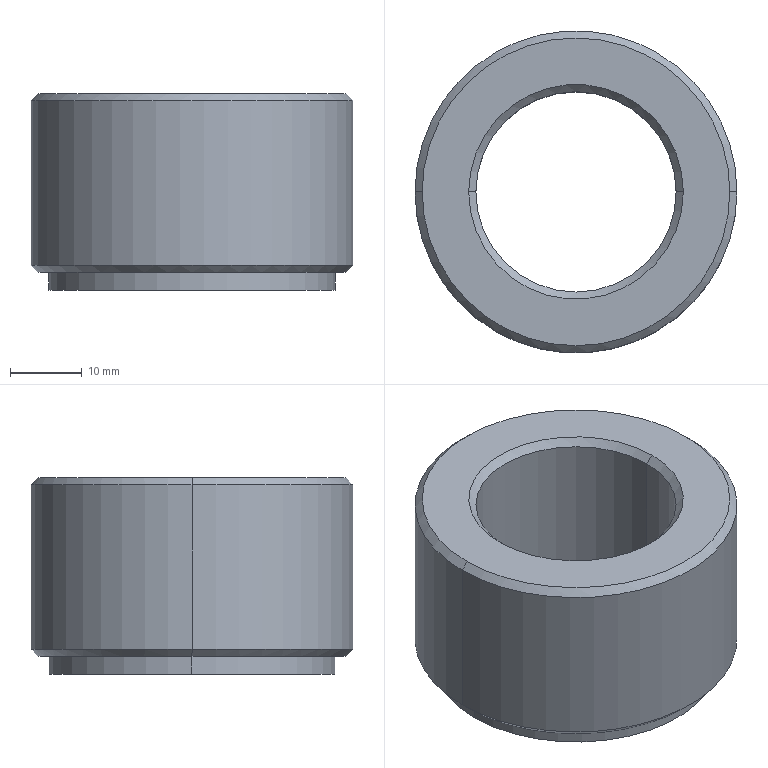Part | SolidWorks | features 3DProfileFeature 1, Chamfer 1, Extrusion 1, HoleWzd 1, ICE 1 | 1 solid | 15 faces | box 45 x 45 x 27.5 mm | volume 25785 mm3 | cone 6 | cylinder 6 | plane 3 | commonest cylinder face diameters 28 x2 40 x2 45 x2
STEP:
#1=CARTESIAN_POINT('',(-83.421,0.,24.));
#2=VERTEX_POINT('',#1);
#3=CARTESIAN_POINT('',(-55.421,0.,24.));
#4=VERTEX_POINT('',#3);
#5=CARTESIAN_POINT('',(-69.421,0.,24.));
#6=DIRECTION('',(0.,0.,1.));
#7=DIRECTION('',(1.,0.,0.));
#8=AXIS2_PLACEMENT_3D('',#5,#6,#7);
#9=CIRCLE('',#8,14.);
#10=EDGE_CURVE('',#2,#4,#9,.T.);
#11=ORIENTED_EDGE('',*,*,#10,.F.);
#12=CARTESIAN_POINT('',(-84.421,0.,25.));
#13=VERTEX_POINT('',#12);
#14=CARTESIAN_POINT('',(-83.421,0.,24.));
#15=DIRECTION('',(-0.7071,0.,0.7071));
#16=VECTOR('',#15,1000.);
#17=LINE('',#14,#16);
#18=EDGE_CURVE('',#2,#13,#17,.T.);
#19=ORIENTED_EDGE('',*,*,#18,.T.);
#20=CARTESIAN_POINT('',(-54.421,0.,25.));
#21=VERTEX_POINT('',#20);
#22=CARTESIAN_POINT('',(-69.421,0.,25.));
#23=DIRECTION('',(0.,0.,-1.));
#24=DIRECTION('',(1.,0.,0.));
#25=AXIS2_PLACEMENT_3D('',#22,#23,#24);
#26=CIRCLE('',#25,15.);
#27=EDGE_CURVE('',#21,#13,#26,.T.);
#28=ORIENTED_EDGE('',*,*,#27,.F.);
#29=CARTESIAN_POINT('',(-55.421,0.,24.));
#30=DIRECTION('',(0.7071,0.,0.7071));
#31=VECTOR('',#30,1000.);
#32=LINE('',#29,#31);
#33=EDGE_CURVE('',#4,#21,#32,.T.);
#34=ORIENTED_EDGE('',*,*,#33,.F.);
#35=EDGE_LOOP('',(#11,#19,#28,#34));
#36=FACE_OUTER_BOUND('',#35,.T.);
#37=CARTESIAN_POINT('',(-69.421,0.,24.));
#38=DIRECTION('',(0.,0.,1.));
#39=DIRECTION('',(1.,0.,0.));
#40=AXIS2_PLACEMENT_3D('',#37,#38,#39);
#41=CONICAL_SURFACE('',#40,14.,0.7854);
#42=ADVANCED_FACE('',(#36),#41,.F.);
#43=CARTESIAN_POINT('',(-47.921,0.,25.));
#44=VERTEX_POINT('',#43);
#45=CARTESIAN_POINT('',(-90.921,0.,25.));
#46=VERTEX_POINT('',#45);
#47=CARTESIAN_POINT('',(-69.421,0.,25.));
#48=DIRECTION('',(0.,0.,1.));
#49=DIRECTION('',(1.,0.,0.));
#50=AXIS2_PLACEMENT_3D('',#47,#48,#49);
#51=CIRCLE('',#50,21.5);
#52=EDGE_CURVE('',#44,#46,#51,.T.);
#53=ORIENTED_EDGE('',*,*,#52,.F.);
#54=CARTESIAN_POINT('',(-46.921,0.,24.));
#55=VERTEX_POINT('',#54);
#56=CARTESIAN_POINT('',(-47.921,0.,25.));
#57=DIRECTION('',(0.7071,0.,-0.7071));
#58=VECTOR('',#57,1000.);
#59=LINE('',#56,#58);
#60=EDGE_CURVE('',#44,#55,#59,.T.);
#61=ORIENTED_EDGE('',*,*,#60,.T.);
#62=CARTESIAN_POINT('',(-91.921,0.,24.));
#63=VERTEX_POINT('',#62);
#64=CARTESIAN_POINT('',(-69.421,0.,24.));
#65=DIRECTION('',(0.,0.,-1.));
#66=DIRECTION('',(1.,0.,0.));
#67=AXIS2_PLACEMENT_3D('',#64,#65,#66);
#68=CIRCLE('',#67,22.5);
#69=EDGE_CURVE('',#63,#55,#68,.T.);
#70=ORIENTED_EDGE('',*,*,#69,.F.);
#71=CARTESIAN_POINT('',(-90.921,0.,25.));
#72=DIRECTION('',(-0.7071,0.,-0.7071));
#73=VECTOR('',#72,1000.);
#74=LINE('',#71,#73);
#75=EDGE_CURVE('',#46,#63,#74,.T.);
#76=ORIENTED_EDGE('',*,*,#75,.F.);
#77=EDGE_LOOP('',(#53,#61,#70,#76));
#78=FACE_OUTER_BOUND('',#77,.T.);
#79=CARTESIAN_POINT('',(-69.421,0.,25.));
#80=DIRECTION('',(0.,0.,-1.));
#81=DIRECTION('',(-1.,0.,0.));
#82=AXIS2_PLACEMENT_3D('',#79,#80,#81);
#83=CONICAL_SURFACE('',#82,21.5,0.7854);
#84=ADVANCED_FACE('',(#78),#83,.T.);
#85=CARTESIAN_POINT('',(-90.921,0.,0.));
#86=VERTEX_POINT('',#85);
#87=CARTESIAN_POINT('',(-47.921,0.,0.));
#88=VERTEX_POINT('',#87);
#89=CARTESIAN_POINT('',(-69.421,0.,0.));
#90=DIRECTION('',(0.,0.,-1.));
#91=DIRECTION('',(1.,0.,0.));
#92=AXIS2_PLACEMENT_3D('',#89,#90,#91);
#93=CIRCLE('',#92,21.5);
#94=EDGE_CURVE('',#86,#88,#93,.T.);
#95=ORIENTED_EDGE('',*,*,#94,.F.);
#96=CARTESIAN_POINT('',(-91.921,0.,1.));
#97=VERTEX_POINT('',#96);
#98=CARTESIAN_POINT('',(-91.921,0.,1.));
#99=DIRECTION('',(-0.7071,0.,0.7071));
#100=VECTOR('',#99,1000.);
#101=LINE('',#98,#100);
#102=EDGE_CURVE('',#86,#97,#101,.T.);
#103=ORIENTED_EDGE('',*,*,#102,.T.);
#104=CARTESIAN_POINT('',(-46.921,0.,1.));
#105=VERTEX_POINT('',#104);
#106=CARTESIAN_POINT('',(-69.421,0.,1.));
#107=DIRECTION('',(0.,0.,1.));
#108=DIRECTION('',(1.,0.,0.));
#109=AXIS2_PLACEMENT_3D('',#106,#107,#108);
#110=CIRCLE('',#109,22.5);
#111=EDGE_CURVE('',#105,#97,#110,.T.);
#112=ORIENTED_EDGE('',*,*,#111,.F.);
#113=CARTESIAN_POINT('',(-46.921,0.,1.));
#114=DIRECTION('',(0.7071,0.,0.7071));
#115=VECTOR('',#114,1000.);
#116=LINE('',#113,#115);
#117=EDGE_CURVE('',#88,#105,#116,.T.);
#118=ORIENTED_EDGE('',*,*,#117,.F.);
#119=EDGE_LOOP('',(#95,#103,#112,#118));
#120=FACE_OUTER_BOUND('',#119,.T.);
#121=CARTESIAN_POINT('',(-69.421,0.,1.));
#122=DIRECTION('',(0.,0.,1.));
#123=DIRECTION('',(1.,0.,0.));
#124=AXIS2_PLACEMENT_3D('',#121,#122,#123);
#125=CONICAL_SURFACE('',#124,22.5,0.7854);
#126=ADVANCED_FACE('',(#120),#125,.T.);
#127=CARTESIAN_POINT('',(-89.421,0.,-2.5));
#128=VERTEX_POINT('',#127);
#129=CARTESIAN_POINT('',(-49.421,0.,-2.5));
#130=VERTEX_POINT('',#129);
#131=CARTESIAN_POINT('',(-69.421,0.,-2.5));
#132=DIRECTION('',(0.,0.,-1.));
#133=DIRECTION('',(-1.,0.,0.));
#134=AXIS2_PLACEMENT_3D('',#131,#132,#133);
#135=CIRCLE('',#134,20.);
#136=EDGE_CURVE('',#128,#130,#135,.T.);
#137=ORIENTED_EDGE('',*,*,#136,.F.);
#138=CARTESIAN_POINT('',(-89.421,0.,0.));
#139=VERTEX_POINT('',#138);
#140=CARTESIAN_POINT('',(-89.421,0.,-2.5));
#141=DIRECTION('',(0.,0.,1.));
#142=VECTOR('',#141,1000.);
#143=LINE('',#140,#142);
#144=EDGE_CURVE('',#128,#139,#143,.T.);
#145=ORIENTED_EDGE('',*,*,#144,.T.);
#146=CARTESIAN_POINT('',(-49.421,0.,0.));
#147=VERTEX_POINT('',#146);
#148=CARTESIAN_POINT('',(-69.421,0.,0.));
#149=DIRECTION('',(0.,0.,-1.));
#150=DIRECTION('',(1.,0.,0.));
#151=AXIS2_PLACEMENT_3D('',#148,#149,#150);
#152=CIRCLE('',#151,20.);
#153=EDGE_CURVE('',#139,#147,#152,.T.);
#154=ORIENTED_EDGE('',*,*,#153,.T.);
#155=CARTESIAN_POINT('',(-49.421,0.,-2.5));
#156=DIRECTION('',(0.,0.,1.));
#157=VECTOR('',#156,1000.);
#158=LINE('',#155,#157);
#159=EDGE_CURVE('',#130,#147,#158,.T.);
#160=ORIENTED_EDGE('',*,*,#159,.F.);
#161=EDGE_LOOP('',(#137,#145,#154,#160));
#162=FACE_OUTER_BOUND('',#161,.T.);
#163=CARTESIAN_POINT('',(-69.421,0.,-2.5));
#164=DIRECTION('',(0.,0.,1.));
#165=DIRECTION('',(1.,0.,0.));
#166=AXIS2_PLACEMENT_3D('',#163,#164,#165);
#167=CYLINDRICAL_SURFACE('',#166,20.);
#168=ADVANCED_FACE('',(#162),#167,.T.);
#169=CARTESIAN_POINT('',(-55.421,0.,-2.5));
#170=VERTEX_POINT('',#169);
#171=CARTESIAN_POINT('',(-83.421,0.,-2.5));
#172=VERTEX_POINT('',#171);
#173=CARTESIAN_POINT('',(-69.421,0.,-2.5));
#174=DIRECTION('',(0.,0.,-1.));
#175=DIRECTION('',(-1.,0.,0.));
#176=AXIS2_PLACEMENT_3D('',#173,#174,#175);
#177=CIRCLE('',#176,14.);
#178=EDGE_CURVE('',#170,#172,#177,.T.);
#179=ORIENTED_EDGE('',*,*,#178,.T.);
#180=CARTESIAN_POINT('',(-83.421,0.,25.));
#181=DIRECTION('',(0.,0.,1.));
#182=VECTOR('',#181,1000.);
#183=LINE('',#180,#182);
#184=EDGE_CURVE('',#172,#2,#183,.T.);
#185=ORIENTED_EDGE('',*,*,#184,.T.);
#186=ORIENTED_EDGE('',*,*,#10,.T.);
#187=CARTESIAN_POINT('',(-55.421,0.,25.));
#188=DIRECTION('',(0.,0.,1.));
#189=VECTOR('',#188,1000.);
#190=LINE('',#187,#189);
#191=EDGE_CURVE('',#170,#4,#190,.T.);
#192=ORIENTED_EDGE('',*,*,#191,.F.);
#193=EDGE_LOOP('',(#179,#185,#186,#192));
#194=FACE_OUTER_BOUND('',#193,.T.);
#195=CARTESIAN_POINT('',(-69.421,0.,25.));
#196=DIRECTION('',(0.,0.,1.));
#197=DIRECTION('',(1.,0.,0.));
#198=AXIS2_PLACEMENT_3D('',#195,#196,#197);
#199=CYLINDRICAL_SURFACE('',#198,14.);
#200=ADVANCED_FACE('',(#194),#199,.F.);
#201=ORIENTED_EDGE('',*,*,#69,.T.);
#202=CARTESIAN_POINT('',(-46.921,0.,25.));
#203=DIRECTION('',(0.,0.,-1.));
#204=VECTOR('',#203,1000.);
#205=LINE('',#202,#204);
#206=EDGE_CURVE('',#55,#105,#205,.T.);
#207=ORIENTED_EDGE('',*,*,#206,.T.);
#208=ORIENTED_EDGE('',*,*,#111,.T.);
#209=CARTESIAN_POINT('',(-91.921,0.,25.));
#210=DIRECTION('',(0.,0.,-1.));
#211=VECTOR('',#210,1000.);
#212=LINE('',#209,#211);
#213=EDGE_CURVE('',#63,#97,#212,.T.);
#214=ORIENTED_EDGE('',*,*,#213,.F.);
#215=EDGE_LOOP('',(#201,#207,#208,#214));
#216=FACE_OUTER_BOUND('',#215,.T.);
#217=CARTESIAN_POINT('',(-69.421,0.,25.));
#218=DIRECTION('',(0.,0.,-1.));
#219=DIRECTION('',(-1.,0.,0.));
#220=AXIS2_PLACEMENT_3D('',#217,#218,#219);
#221=CYLINDRICAL_SURFACE('',#220,22.5);
#222=ADVANCED_FACE('',(#216),#221,.T.);
#223=CARTESIAN_POINT('',(-69.421,0.,0.));
#224=DIRECTION('',(0.,0.,-1.));
#225=DIRECTION('',(1.,0.,0.));
#226=AXIS2_PLACEMENT_3D('',#223,#224,#225);
#227=CIRCLE('',#226,21.5);
#228=EDGE_CURVE('',#88,#86,#227,.T.);
#229=ORIENTED_EDGE('',*,*,#228,.T.);
#230=ORIENTED_EDGE('',*,*,#94,.T.);
#231=EDGE_LOOP('',(#229,#230));
#232=FACE_OUTER_BOUND('',#231,.T.);
#233=CARTESIAN_POINT('',(-69.421,0.,0.));
#234=DIRECTION('',(0.,0.,-1.));
#235=DIRECTION('',(1.,0.,0.));
#236=AXIS2_PLACEMENT_3D('',#233,#234,#235);
#237=CIRCLE('',#236,20.);
#238=EDGE_CURVE('',#147,#139,#237,.T.);
#239=ORIENTED_EDGE('',*,*,#238,.F.);
#240=ORIENTED_EDGE('',*,*,#153,.F.);
#241=EDGE_LOOP('',(#239,#240));
#242=FACE_BOUND('',#241,.T.);
#243=CARTESIAN_POINT('',(-69.421,0.,0.));
#244=DIRECTION('',(0.,0.,1.));
#245=DIRECTION('',(1.,0.,0.));
#246=AXIS2_PLACEMENT_3D('',#243,#244,#245);
#247=PLANE('',#246);
#248=ADVANCED_FACE('',(#232,#242),#247,.F.);
#249=ORIENTED_EDGE('',*,*,#206,.F.);
#250=CARTESIAN_POINT('',(-69.421,0.,24.));
#251=DIRECTION('',(0.,0.,-1.));
#252=DIRECTION('',(1.,0.,0.));
#253=AXIS2_PLACEMENT_3D('',#250,#251,#252);
#254=CIRCLE('',#253,22.5);
#255=EDGE_CURVE('',#55,#63,#254,.T.);
#256=ORIENTED_EDGE('',*,*,#255,.T.);
#257=ORIENTED_EDGE('',*,*,#213,.T.);
#258=CARTESIAN_POINT('',(-69.421,0.,1.));
#259=DIRECTION('',(0.,0.,1.));
#260=DIRECTION('',(1.,0.,0.));
#261=AXIS2_PLACEMENT_3D('',#258,#259,#260);
#262=CIRCLE('',#261,22.5);
#263=EDGE_CURVE('',#97,#105,#262,.T.);
#264=ORIENTED_EDGE('',*,*,#263,.T.);
#265=EDGE_LOOP('',(#249,#256,#257,#264));
#266=FACE_OUTER_BOUND('',#265,.T.);
#267=CARTESIAN_POINT('',(-69.421,0.,25.));
#268=DIRECTION('',(0.,0.,-1.));
#269=DIRECTION('',(-1.,0.,0.));
#270=AXIS2_PLACEMENT_3D('',#267,#268,#269);
#271=CYLINDRICAL_SURFACE('',#270,22.5);
#272=ADVANCED_FACE('',(#266),#271,.T.);
#273=CARTESIAN_POINT('',(-69.421,0.,25.));
#274=DIRECTION('',(0.,0.,1.));
#275=DIRECTION('',(1.,0.,0.));
#276=AXIS2_PLACEMENT_3D('',#273,#274,#275);
#277=CIRCLE('',#276,21.5);
#278=EDGE_CURVE('',#46,#44,#277,.T.);
#279=ORIENTED_EDGE('',*,*,#278,.T.);
#280=ORIENTED_EDGE('',*,*,#52,.T.);
#281=EDGE_LOOP('',(#279,#280));
#282=FACE_OUTER_BOUND('',#281,.T.);
#283=ORIENTED_EDGE('',*,*,#27,.T.);
#284=CARTESIAN_POINT('',(-69.421,0.,25.));
#285=DIRECTION('',(0.,0.,-1.));
#286=DIRECTION('',(1.,0.,0.));
#287=AXIS2_PLACEMENT_3D('',#284,#285,#286);
#288=CIRCLE('',#287,15.);
#289=EDGE_CURVE('',#13,#21,#288,.T.);
#290=ORIENTED_EDGE('',*,*,#289,.T.);
#291=EDGE_LOOP('',(#283,#290));
#292=FACE_BOUND('',#291,.T.);
#293=CARTESIAN_POINT('',(-69.421,0.,25.));
#294=DIRECTION('',(0.,0.,1.));
#295=DIRECTION('',(1.,0.,0.));
#296=AXIS2_PLACEMENT_3D('',#293,#294,#295);
#297=PLANE('',#296);
#298=ADVANCED_FACE('',(#282,#292),#297,.T.);
#299=ORIENTED_EDGE('',*,*,#184,.F.);
#300=CARTESIAN_POINT('',(-69.421,0.,-2.5));
#301=DIRECTION('',(0.,0.,-1.));
#302=DIRECTION('',(-1.,0.,0.));
#303=AXIS2_PLACEMENT_3D('',#300,#301,#302);
#304=CIRCLE('',#303,14.);
#305=EDGE_CURVE('',#172,#170,#304,.T.);
#306=ORIENTED_EDGE('',*,*,#305,.T.);
#307=ORIENTED_EDGE('',*,*,#191,.T.);
#308=CARTESIAN_POINT('',(-69.421,0.,24.));
#309=DIRECTION('',(0.,0.,1.));
#310=DIRECTION('',(1.,0.,0.));
#311=AXIS2_PLACEMENT_3D('',#308,#309,#310);
#312=CIRCLE('',#311,14.);
#313=EDGE_CURVE('',#4,#2,#312,.T.);
#314=ORIENTED_EDGE('',*,*,#313,.T.);
#315=EDGE_LOOP('',(#299,#306,#307,#314));
#316=FACE_OUTER_BOUND('',#315,.T.);
#317=CARTESIAN_POINT('',(-69.421,0.,25.));
#318=DIRECTION('',(0.,0.,1.));
#319=DIRECTION('',(1.,0.,0.));
#320=AXIS2_PLACEMENT_3D('',#317,#318,#319);
#321=CYLINDRICAL_SURFACE('',#320,14.);
#322=ADVANCED_FACE('',(#316),#321,.F.);
#323=CARTESIAN_POINT('',(-69.421,0.,-2.5));
#324=DIRECTION('',(0.,0.,-1.));
#325=DIRECTION('',(-1.,0.,0.));
#326=AXIS2_PLACEMENT_3D('',#323,#324,#325);
#327=CIRCLE('',#326,20.);
#328=EDGE_CURVE('',#130,#128,#327,.T.);
#329=ORIENTED_EDGE('',*,*,#328,.T.);
#330=ORIENTED_EDGE('',*,*,#136,.T.);
#331=EDGE_LOOP('',(#329,#330));
#332=FACE_OUTER_BOUND('',#331,.T.);
#333=ORIENTED_EDGE('',*,*,#178,.F.);
#334=ORIENTED_EDGE('',*,*,#305,.F.);
#335=EDGE_LOOP('',(#333,#334));
#336=FACE_BOUND('',#335,.T.);
#337=CARTESIAN_POINT('',(-69.421,0.,-2.5));
#338=DIRECTION('',(0.,0.,-1.));
#339=DIRECTION('',(-1.,0.,0.));
#340=AXIS2_PLACEMENT_3D('',#337,#338,#339);
#341=PLANE('',#340);
#342=ADVANCED_FACE('',(#332,#336),#341,.T.);
#343=ORIENTED_EDGE('',*,*,#144,.F.);
#344=ORIENTED_EDGE('',*,*,#328,.F.);
#345=ORIENTED_EDGE('',*,*,#159,.T.);
#346=ORIENTED_EDGE('',*,*,#238,.T.);
#347=EDGE_LOOP('',(#343,#344,#345,#346));
#348=FACE_OUTER_BOUND('',#347,.T.);
#349=CARTESIAN_POINT('',(-69.421,0.,-2.5));
#350=DIRECTION('',(0.,0.,1.));
#351=DIRECTION('',(1.,0.,0.));
#352=AXIS2_PLACEMENT_3D('',#349,#350,#351);
#353=CYLINDRICAL_SURFACE('',#352,20.);
#354=ADVANCED_FACE('',(#348),#353,.T.);
#355=ORIENTED_EDGE('',*,*,#102,.F.);
#356=ORIENTED_EDGE('',*,*,#228,.F.);
#357=ORIENTED_EDGE('',*,*,#117,.T.);
#358=ORIENTED_EDGE('',*,*,#263,.F.);
#359=EDGE_LOOP('',(#355,#356,#357,#358));
#360=FACE_OUTER_BOUND('',#359,.T.);
#361=CARTESIAN_POINT('',(-69.421,0.,1.));
#362=DIRECTION('',(0.,0.,1.));
#363=DIRECTION('',(1.,0.,0.));
#364=AXIS2_PLACEMENT_3D('',#361,#362,#363);
#365=CONICAL_SURFACE('',#364,22.5,0.7854);
#366=ADVANCED_FACE('',(#360),#365,.T.);
#367=ORIENTED_EDGE('',*,*,#60,.F.);
#368=ORIENTED_EDGE('',*,*,#278,.F.);
#369=ORIENTED_EDGE('',*,*,#75,.T.);
#370=ORIENTED_EDGE('',*,*,#255,.F.);
#371=EDGE_LOOP('',(#367,#368,#369,#370));
#372=FACE_OUTER_BOUND('',#371,.T.);
#373=CARTESIAN_POINT('',(-69.421,0.,25.));
#374=DIRECTION('',(0.,0.,-1.));
#375=DIRECTION('',(-1.,0.,0.));
#376=AXIS2_PLACEMENT_3D('',#373,#374,#375);
#377=CONICAL_SURFACE('',#376,21.5,0.7854);
#378=ADVANCED_FACE('',(#372),#377,.T.);
#379=ORIENTED_EDGE('',*,*,#18,.F.);
#380=ORIENTED_EDGE('',*,*,#313,.F.);
#381=ORIENTED_EDGE('',*,*,#33,.T.);
#382=ORIENTED_EDGE('',*,*,#289,.F.);
#383=EDGE_LOOP('',(#379,#380,#381,#382));
#384=FACE_OUTER_BOUND('',#383,.T.);
#385=CARTESIAN_POINT('',(-69.421,0.,24.));
#386=DIRECTION('',(0.,0.,1.));
#387=DIRECTION('',(1.,0.,0.));
#388=AXIS2_PLACEMENT_3D('',#385,#386,#387);
#389=CONICAL_SURFACE('',#388,14.,0.7854);
#390=ADVANCED_FACE('',(#384),#389,.F.);
#391=CLOSED_SHELL('',(#42,#84,#126,#168,#200,#222,#248,#272,#298,#322,#342,#354,#366,#378,#390));
#392=MANIFOLD_SOLID_BREP('',#391);
#393=CARTESIAN_POINT('',(0.,0.,0.));
#394=DIRECTION('',(0.,0.,1.));
#395=DIRECTION('',(1.,0.,0.));
#396=AXIS2_PLACEMENT_3D('',#393,#394,#395);
#397=(LENGTH_UNIT()NAMED_UNIT(*)SI_UNIT(.MILLI.,.METRE.));
#398=UNCERTAINTY_MEASURE_WITH_UNIT(LENGTH_MEASURE(0.00001),#397,'','');
#399=(NAMED_UNIT(*)PLANE_ANGLE_UNIT()SI_UNIT($,.RADIAN.));
#400=(NAMED_UNIT(*)SI_UNIT($,.STERADIAN.)SOLID_ANGLE_UNIT());
#401=(GEOMETRIC_REPRESENTATION_CONTEXT(3)GLOBAL_UNCERTAINTY_ASSIGNED_CONTEXT((#398))GLOBAL_UNIT_ASSIGNED_CONTEXT((#397,#399,#400))REPRESENTATION_CONTEXT('',''));
#402=ADVANCED_BREP_SHAPE_REPRESENTATION('',(#392,#396),#401);